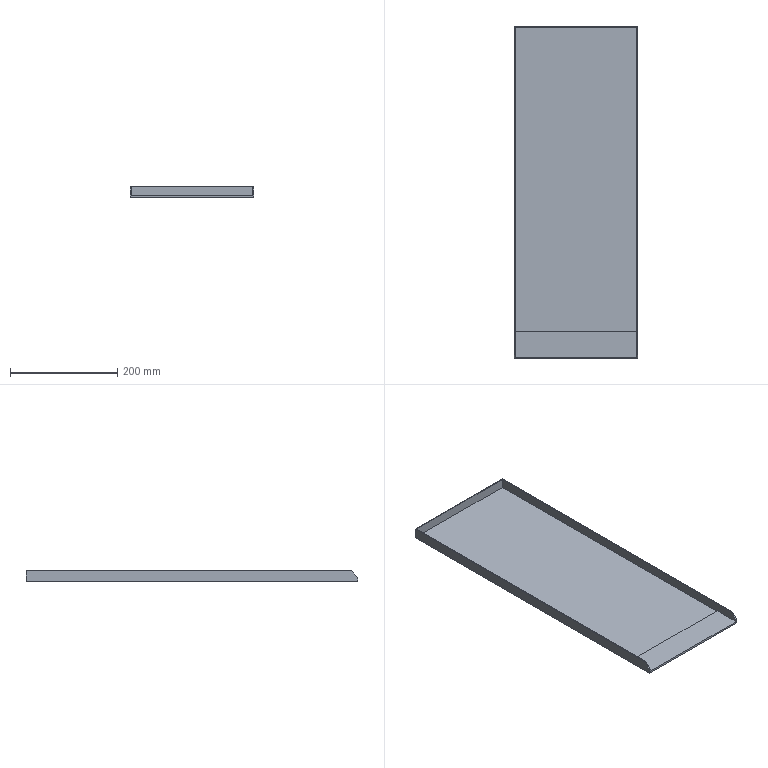Part | NX | features solid 2 | 1 solid | 14 faces | box 230 x 620 x 20 mm | volume 360238 mm3 | plane 14
STEP:
#1=CARTESIAN_POINT('',(360.,-460.,-313.));
#2=VERTEX_POINT('',#1);
#3=CARTESIAN_POINT('',(360.,-460.,-320.));
#4=VERTEX_POINT('',#3);
#5=CARTESIAN_POINT('',(360.,-460.,-318.));
#6=DIRECTION('',(0.,0.,-1.));
#7=VECTOR('',#6,1000.);
#8=LINE('',#5,#7);
#9=EDGE_CURVE('',#2,#4,#8,.T.);
#10=ORIENTED_EDGE('',*,*,#9,.F.);
#11=CARTESIAN_POINT('',(360.,-447.,-300.));
#12=VERTEX_POINT('',#11);
#13=CARTESIAN_POINT('',(360.,-445.,-298.));
#14=DIRECTION('',(0.,0.7071,0.7071));
#15=VECTOR('',#14,1000.);
#16=LINE('',#13,#15);
#17=EDGE_CURVE('',#2,#12,#16,.T.);
#18=ORIENTED_EDGE('',*,*,#17,.T.);
#19=CARTESIAN_POINT('',(360.,160.,-300.));
#20=VERTEX_POINT('',#19);
#21=CARTESIAN_POINT('',(360.,-70.,-300.));
#22=DIRECTION('',(0.,-1.,0.));
#23=VECTOR('',#22,1000.);
#24=LINE('',#21,#23);
#25=EDGE_CURVE('',#20,#12,#24,.T.);
#26=ORIENTED_EDGE('',*,*,#25,.F.);
#27=CARTESIAN_POINT('',(360.,160.,-320.));
#28=VERTEX_POINT('',#27);
#29=CARTESIAN_POINT('',(360.,160.,-318.));
#30=DIRECTION('',(0.,0.,-1.));
#31=VECTOR('',#30,1000.);
#32=LINE('',#29,#31);
#33=EDGE_CURVE('',#20,#28,#32,.T.);
#34=ORIENTED_EDGE('',*,*,#33,.T.);
#35=CARTESIAN_POINT('',(360.,-70.,-320.));
#36=DIRECTION('',(0.,1.,0.));
#37=VECTOR('',#36,1000.);
#38=LINE('',#35,#37);
#39=EDGE_CURVE('',#28,#4,#38,.F.);
#40=ORIENTED_EDGE('',*,*,#39,.T.);
#41=EDGE_LOOP('',(#10,#18,#26,#34,#40));
#42=FACE_BOUND('',#41,.T.);
#43=CARTESIAN_POINT('',(360.,-70.,-318.));
#44=DIRECTION('',(1.,0.,0.));
#45=DIRECTION('',(0.,0.,-1.));
#46=AXIS2_PLACEMENT_3D('',#43,#44,#45);
#47=PLANE('',#46);
#48=ADVANCED_FACE('',(#42),#47,.F.);
#49=CARTESIAN_POINT('',(590.,160.,-320.));
#50=VERTEX_POINT('',#49);
#51=CARTESIAN_POINT('',(-350.,160.,-320.));
#52=DIRECTION('',(1.,0.,0.));
#53=VECTOR('',#52,1000.);
#54=LINE('',#51,#53);
#55=EDGE_CURVE('',#50,#28,#54,.F.);
#56=ORIENTED_EDGE('',*,*,#55,.T.);
#57=ORIENTED_EDGE('',*,*,#33,.F.);
#58=CARTESIAN_POINT('',(590.,160.,-300.));
#59=VERTEX_POINT('',#58);
#60=CARTESIAN_POINT('',(-380.,160.,-300.));
#61=DIRECTION('',(1.,0.,0.));
#62=VECTOR('',#61,1000.);
#63=LINE('',#60,#62);
#64=EDGE_CURVE('',#20,#59,#63,.T.);
#65=ORIENTED_EDGE('',*,*,#64,.T.);
#66=CARTESIAN_POINT('',(590.,160.,-318.));
#67=DIRECTION('',(0.,0.,-1.));
#68=VECTOR('',#67,1000.);
#69=LINE('',#66,#68);
#70=EDGE_CURVE('',#59,#50,#69,.T.);
#71=ORIENTED_EDGE('',*,*,#70,.T.);
#72=EDGE_LOOP('',(#56,#57,#65,#71));
#73=FACE_BOUND('',#72,.T.);
#74=CARTESIAN_POINT('',(-350.,160.,-318.));
#75=DIRECTION('',(0.,-1.,0.));
#76=DIRECTION('',(0.,0.,-1.));
#77=AXIS2_PLACEMENT_3D('',#74,#75,#76);
#78=PLANE('',#77);
#79=ADVANCED_FACE('',(#73),#78,.F.);
#80=CARTESIAN_POINT('',(590.,-447.,-300.));
#81=VERTEX_POINT('',#80);
#82=CARTESIAN_POINT('',(590.,-15.,-300.));
#83=DIRECTION('',(0.,-1.,0.));
#84=VECTOR('',#83,1000.);
#85=LINE('',#82,#84);
#86=EDGE_CURVE('',#59,#81,#85,.T.);
#87=ORIENTED_EDGE('',*,*,#86,.T.);
#88=CARTESIAN_POINT('',(590.,-460.,-313.));
#89=VERTEX_POINT('',#88);
#90=CARTESIAN_POINT('',(590.,-460.,-313.));
#91=DIRECTION('',(0.,-0.7071,-0.7071));
#92=VECTOR('',#91,1000.);
#93=LINE('',#90,#92);
#94=EDGE_CURVE('',#81,#89,#93,.T.);
#95=ORIENTED_EDGE('',*,*,#94,.T.);
#96=CARTESIAN_POINT('',(590.,-460.,-320.));
#97=VERTEX_POINT('',#96);
#98=CARTESIAN_POINT('',(590.,-460.,-318.));
#99=DIRECTION('',(0.,0.,-1.));
#100=VECTOR('',#99,1000.);
#101=LINE('',#98,#100);
#102=EDGE_CURVE('',#89,#97,#101,.T.);
#103=ORIENTED_EDGE('',*,*,#102,.T.);
#104=CARTESIAN_POINT('',(590.,-70.,-320.));
#105=DIRECTION('',(0.,-1.,0.));
#106=VECTOR('',#105,1000.);
#107=LINE('',#104,#106);
#108=EDGE_CURVE('',#97,#50,#107,.F.);
#109=ORIENTED_EDGE('',*,*,#108,.T.);
#110=ORIENTED_EDGE('',*,*,#70,.F.);
#111=EDGE_LOOP('',(#87,#95,#103,#109,#110));
#112=FACE_BOUND('',#111,.T.);
#113=CARTESIAN_POINT('',(590.,-70.,-318.));
#114=DIRECTION('',(-1.,0.,0.));
#115=DIRECTION('',(0.,0.,1.));
#116=AXIS2_PLACEMENT_3D('',#113,#114,#115);
#117=PLANE('',#116);
#118=ADVANCED_FACE('',(#112),#117,.F.);
#119=CARTESIAN_POINT('',(362.,-460.,-316.));
#120=VERTEX_POINT('',#119);
#121=CARTESIAN_POINT('',(588.,-460.,-316.));
#122=VERTEX_POINT('',#121);
#123=CARTESIAN_POINT('',(362.,-460.,-316.));
#124=DIRECTION('',(-1.,0.,0.));
#125=VECTOR('',#124,1000.);
#126=LINE('',#123,#125);
#127=EDGE_CURVE('',#120,#122,#126,.F.);
#128=ORIENTED_EDGE('',*,*,#127,.F.);
#129=CARTESIAN_POINT('',(362.,-460.,-313.));
#130=VERTEX_POINT('',#129);
#131=CARTESIAN_POINT('',(362.,-460.,-318.));
#132=DIRECTION('',(0.,0.,-1.));
#133=VECTOR('',#132,1000.);
#134=LINE('',#131,#133);
#135=EDGE_CURVE('',#130,#120,#134,.T.);
#136=ORIENTED_EDGE('',*,*,#135,.F.);
#137=CARTESIAN_POINT('',(360.,-460.,-313.));
#138=DIRECTION('',(-1.,0.,0.));
#139=VECTOR('',#138,1000.);
#140=LINE('',#137,#139);
#141=EDGE_CURVE('',#130,#2,#140,.T.);
#142=ORIENTED_EDGE('',*,*,#141,.T.);
#143=ORIENTED_EDGE('',*,*,#9,.T.);
#144=CARTESIAN_POINT('',(-350.,-460.,-320.));
#145=DIRECTION('',(-1.,0.,0.));
#146=VECTOR('',#145,1000.);
#147=LINE('',#144,#146);
#148=EDGE_CURVE('',#4,#97,#147,.F.);
#149=ORIENTED_EDGE('',*,*,#148,.T.);
#150=ORIENTED_EDGE('',*,*,#102,.F.);
#151=CARTESIAN_POINT('',(588.,-460.,-313.));
#152=VERTEX_POINT('',#151);
#153=CARTESIAN_POINT('',(588.,-460.,-313.));
#154=DIRECTION('',(-1.,0.,0.));
#155=VECTOR('',#154,1000.);
#156=LINE('',#153,#155);
#157=EDGE_CURVE('',#89,#152,#156,.T.);
#158=ORIENTED_EDGE('',*,*,#157,.T.);
#159=CARTESIAN_POINT('',(588.,-460.,-318.));
#160=DIRECTION('',(0.,0.,-1.));
#161=VECTOR('',#160,1000.);
#162=LINE('',#159,#161);
#163=EDGE_CURVE('',#152,#122,#162,.T.);
#164=ORIENTED_EDGE('',*,*,#163,.T.);
#165=EDGE_LOOP('',(#128,#136,#142,#143,#149,#150,#158,#164));
#166=FACE_BOUND('',#165,.T.);
#167=CARTESIAN_POINT('',(-350.,-460.,-318.));
#168=DIRECTION('',(0.,1.,0.));
#169=DIRECTION('',(0.,0.,1.));
#170=AXIS2_PLACEMENT_3D('',#167,#168,#169);
#171=PLANE('',#170);
#172=ADVANCED_FACE('',(#166),#171,.F.);
#173=CARTESIAN_POINT('',(362.,-410.,-318.));
#174=VERTEX_POINT('',#173);
#175=CARTESIAN_POINT('',(588.,-410.,-318.));
#176=VERTEX_POINT('',#175);
#177=CARTESIAN_POINT('',(362.,-410.,-318.));
#178=DIRECTION('',(1.,0.,0.));
#179=VECTOR('',#178,1000.);
#180=LINE('',#177,#179);
#181=EDGE_CURVE('',#174,#176,#180,.T.);
#182=ORIENTED_EDGE('',*,*,#181,.T.);
#183=CARTESIAN_POINT('',(588.,158.,-318.));
#184=VERTEX_POINT('',#183);
#185=CARTESIAN_POINT('',(588.,-70.,-318.));
#186=DIRECTION('',(0.,1.,0.));
#187=VECTOR('',#186,1000.);
#188=LINE('',#185,#187);
#189=EDGE_CURVE('',#184,#176,#188,.F.);
#190=ORIENTED_EDGE('',*,*,#189,.F.);
#191=CARTESIAN_POINT('',(362.,158.,-318.));
#192=VERTEX_POINT('',#191);
#193=CARTESIAN_POINT('',(-350.,158.,-318.));
#194=DIRECTION('',(-1.,0.,0.));
#195=VECTOR('',#194,1000.);
#196=LINE('',#193,#195);
#197=EDGE_CURVE('',#192,#184,#196,.F.);
#198=ORIENTED_EDGE('',*,*,#197,.F.);
#199=CARTESIAN_POINT('',(362.,-70.,-318.));
#200=DIRECTION('',(0.,-1.,0.));
#201=VECTOR('',#200,1000.);
#202=LINE('',#199,#201);
#203=EDGE_CURVE('',#174,#192,#202,.F.);
#204=ORIENTED_EDGE('',*,*,#203,.F.);
#205=EDGE_LOOP('',(#182,#190,#198,#204));
#206=FACE_BOUND('',#205,.T.);
#207=CARTESIAN_POINT('',(-350.,-70.,-318.));
#208=DIRECTION('',(0.,0.,-1.));
#209=DIRECTION('',(-1.,0.,0.));
#210=AXIS2_PLACEMENT_3D('',#207,#208,#209);
#211=PLANE('',#210);
#212=ADVANCED_FACE('',(#206),#211,.F.);
#213=ORIENTED_EDGE('',*,*,#108,.F.);
#214=ORIENTED_EDGE('',*,*,#148,.F.);
#215=ORIENTED_EDGE('',*,*,#39,.F.);
#216=ORIENTED_EDGE('',*,*,#55,.F.);
#217=EDGE_LOOP('',(#213,#214,#215,#216));
#218=FACE_BOUND('',#217,.T.);
#219=CARTESIAN_POINT('',(-350.,-70.,-320.));
#220=DIRECTION('',(0.,0.,-1.));
#221=DIRECTION('',(-1.,0.,0.));
#222=AXIS2_PLACEMENT_3D('',#219,#220,#221);
#223=PLANE('',#222);
#224=ADVANCED_FACE('',(#218),#223,.T.);
#225=CARTESIAN_POINT('',(588.,-447.,-300.));
#226=VERTEX_POINT('',#225);
#227=CARTESIAN_POINT('',(588.,158.,-300.));
#228=VERTEX_POINT('',#227);
#229=CARTESIAN_POINT('',(588.,-70.,-300.));
#230=DIRECTION('',(0.,1.,0.));
#231=VECTOR('',#230,1000.);
#232=LINE('',#229,#231);
#233=EDGE_CURVE('',#226,#228,#232,.T.);
#234=ORIENTED_EDGE('',*,*,#233,.F.);
#235=CARTESIAN_POINT('',(-380.,-447.,-300.));
#236=DIRECTION('',(1.,0.,0.));
#237=VECTOR('',#236,1000.);
#238=LINE('',#235,#237);
#239=EDGE_CURVE('',#226,#81,#238,.T.);
#240=ORIENTED_EDGE('',*,*,#239,.T.);
#241=ORIENTED_EDGE('',*,*,#86,.F.);
#242=ORIENTED_EDGE('',*,*,#64,.F.);
#243=ORIENTED_EDGE('',*,*,#25,.T.);
#244=CARTESIAN_POINT('',(362.,-447.,-300.));
#245=VERTEX_POINT('',#244);
#246=CARTESIAN_POINT('',(-380.,-447.,-300.));
#247=DIRECTION('',(1.,0.,0.));
#248=VECTOR('',#247,1000.);
#249=LINE('',#246,#248);
#250=EDGE_CURVE('',#12,#245,#249,.T.);
#251=ORIENTED_EDGE('',*,*,#250,.T.);
#252=CARTESIAN_POINT('',(362.,158.,-300.));
#253=VERTEX_POINT('',#252);
#254=CARTESIAN_POINT('',(362.,-70.,-300.));
#255=DIRECTION('',(0.,-1.,0.));
#256=VECTOR('',#255,1000.);
#257=LINE('',#254,#256);
#258=EDGE_CURVE('',#253,#245,#257,.T.);
#259=ORIENTED_EDGE('',*,*,#258,.F.);
#260=CARTESIAN_POINT('',(-350.,158.,-300.));
#261=DIRECTION('',(-1.,0.,0.));
#262=VECTOR('',#261,1000.);
#263=LINE('',#260,#262);
#264=EDGE_CURVE('',#228,#253,#263,.T.);
#265=ORIENTED_EDGE('',*,*,#264,.F.);
#266=EDGE_LOOP('',(#234,#240,#241,#242,#243,#251,#259,#265));
#267=FACE_BOUND('',#266,.T.);
#268=CARTESIAN_POINT('',(-380.,-15.,-300.));
#269=DIRECTION('',(0.,0.,1.));
#270=DIRECTION('',(1.,0.,0.));
#271=AXIS2_PLACEMENT_3D('',#268,#269,#270);
#272=PLANE('',#271);
#273=ADVANCED_FACE('',(#267),#272,.T.);
#274=CARTESIAN_POINT('',(362.,-410.,-316.));
#275=VERTEX_POINT('',#274);
#276=CARTESIAN_POINT('',(362.,-410.,-318.));
#277=DIRECTION('',(0.,0.,1.));
#278=VECTOR('',#277,1000.);
#279=LINE('',#276,#278);
#280=EDGE_CURVE('',#174,#275,#279,.T.);
#281=ORIENTED_EDGE('',*,*,#280,.F.);
#282=ORIENTED_EDGE('',*,*,#203,.T.);
#283=CARTESIAN_POINT('',(362.,158.,-318.));
#284=DIRECTION('',(0.,0.,-1.));
#285=VECTOR('',#284,1000.);
#286=LINE('',#283,#285);
#287=EDGE_CURVE('',#253,#192,#286,.T.);
#288=ORIENTED_EDGE('',*,*,#287,.F.);
#289=ORIENTED_EDGE('',*,*,#258,.T.);
#290=CARTESIAN_POINT('',(362.,-267.5,-120.5));
#291=DIRECTION('',(0.,-0.7071,-0.7071));
#292=VECTOR('',#291,1000.);
#293=LINE('',#290,#292);
#294=EDGE_CURVE('',#245,#130,#293,.T.);
#295=ORIENTED_EDGE('',*,*,#294,.T.);
#296=ORIENTED_EDGE('',*,*,#135,.T.);
#297=CARTESIAN_POINT('',(362.,-410.,-316.));
#298=DIRECTION('',(0.,1.,0.));
#299=VECTOR('',#298,1000.);
#300=LINE('',#297,#299);
#301=EDGE_CURVE('',#275,#120,#300,.F.);
#302=ORIENTED_EDGE('',*,*,#301,.F.);
#303=EDGE_LOOP('',(#281,#282,#288,#289,#295,#296,#302));
#304=FACE_BOUND('',#303,.T.);
#305=CARTESIAN_POINT('',(362.,-70.,-318.));
#306=DIRECTION('',(1.,0.,0.));
#307=DIRECTION('',(0.,0.,-1.));
#308=AXIS2_PLACEMENT_3D('',#305,#306,#307);
#309=PLANE('',#308);
#310=ADVANCED_FACE('',(#304),#309,.T.);
#311=ORIENTED_EDGE('',*,*,#287,.T.);
#312=ORIENTED_EDGE('',*,*,#197,.T.);
#313=CARTESIAN_POINT('',(588.,158.,-318.));
#314=DIRECTION('',(0.,0.,-1.));
#315=VECTOR('',#314,1000.);
#316=LINE('',#313,#315);
#317=EDGE_CURVE('',#228,#184,#316,.T.);
#318=ORIENTED_EDGE('',*,*,#317,.F.);
#319=ORIENTED_EDGE('',*,*,#264,.T.);
#320=EDGE_LOOP('',(#311,#312,#318,#319));
#321=FACE_BOUND('',#320,.T.);
#322=CARTESIAN_POINT('',(-350.,158.,-318.));
#323=DIRECTION('',(0.,-1.,0.));
#324=DIRECTION('',(0.,0.,-1.));
#325=AXIS2_PLACEMENT_3D('',#322,#323,#324);
#326=PLANE('',#325);
#327=ADVANCED_FACE('',(#321),#326,.T.);
#328=CARTESIAN_POINT('',(588.,-410.,-316.));
#329=VERTEX_POINT('',#328);
#330=CARTESIAN_POINT('',(588.,-410.,-318.));
#331=DIRECTION('',(0.,0.,1.));
#332=VECTOR('',#331,1000.);
#333=LINE('',#330,#332);
#334=EDGE_CURVE('',#176,#329,#333,.T.);
#335=ORIENTED_EDGE('',*,*,#334,.T.);
#336=CARTESIAN_POINT('',(588.,-410.,-316.));
#337=DIRECTION('',(0.,1.,0.));
#338=VECTOR('',#337,1000.);
#339=LINE('',#336,#338);
#340=EDGE_CURVE('',#329,#122,#339,.F.);
#341=ORIENTED_EDGE('',*,*,#340,.T.);
#342=ORIENTED_EDGE('',*,*,#163,.F.);
#343=CARTESIAN_POINT('',(588.,-267.5,-120.5));
#344=DIRECTION('',(0.,0.7071,0.7071));
#345=VECTOR('',#344,1000.);
#346=LINE('',#343,#345);
#347=EDGE_CURVE('',#152,#226,#346,.T.);
#348=ORIENTED_EDGE('',*,*,#347,.T.);
#349=ORIENTED_EDGE('',*,*,#233,.T.);
#350=ORIENTED_EDGE('',*,*,#317,.T.);
#351=ORIENTED_EDGE('',*,*,#189,.T.);
#352=EDGE_LOOP('',(#335,#341,#342,#348,#349,#350,#351));
#353=FACE_BOUND('',#352,.T.);
#354=CARTESIAN_POINT('',(588.,-70.,-318.));
#355=DIRECTION('',(-1.,0.,0.));
#356=DIRECTION('',(0.,0.,1.));
#357=AXIS2_PLACEMENT_3D('',#354,#355,#356);
#358=PLANE('',#357);
#359=ADVANCED_FACE('',(#353),#358,.T.);
#360=ORIENTED_EDGE('',*,*,#94,.F.);
#361=ORIENTED_EDGE('',*,*,#239,.F.);
#362=ORIENTED_EDGE('',*,*,#347,.F.);
#363=ORIENTED_EDGE('',*,*,#157,.F.);
#364=EDGE_LOOP('',(#360,#361,#362,#363));
#365=FACE_BOUND('',#364,.T.);
#366=CARTESIAN_POINT('',(-350.,-460.,-313.));
#367=DIRECTION('',(0.,-0.7071,0.7071));
#368=DIRECTION('',(0.,-0.7071,-0.7071));
#369=AXIS2_PLACEMENT_3D('',#366,#367,#368);
#370=PLANE('',#369);
#371=ADVANCED_FACE('',(#365),#370,.T.);
#372=ORIENTED_EDGE('',*,*,#17,.F.);
#373=ORIENTED_EDGE('',*,*,#141,.F.);
#374=ORIENTED_EDGE('',*,*,#294,.F.);
#375=ORIENTED_EDGE('',*,*,#250,.F.);
#376=EDGE_LOOP('',(#372,#373,#374,#375));
#377=FACE_BOUND('',#376,.T.);
#378=CARTESIAN_POINT('',(360.,-445.,-298.));
#379=DIRECTION('',(0.,-0.7071,0.7071));
#380=DIRECTION('',(0.,-0.7071,-0.7071));
#381=AXIS2_PLACEMENT_3D('',#378,#379,#380);
#382=PLANE('',#381);
#383=ADVANCED_FACE('',(#377),#382,.T.);
#384=ORIENTED_EDGE('',*,*,#334,.F.);
#385=ORIENTED_EDGE('',*,*,#181,.F.);
#386=ORIENTED_EDGE('',*,*,#280,.T.);
#387=CARTESIAN_POINT('',(362.,-410.,-316.));
#388=DIRECTION('',(-1.,0.,0.));
#389=VECTOR('',#388,1000.);
#390=LINE('',#387,#389);
#391=EDGE_CURVE('',#275,#329,#390,.F.);
#392=ORIENTED_EDGE('',*,*,#391,.T.);
#393=EDGE_LOOP('',(#384,#385,#386,#392));
#394=FACE_BOUND('',#393,.T.);
#395=CARTESIAN_POINT('',(362.,-410.,-318.));
#396=DIRECTION('',(0.,1.,0.));
#397=DIRECTION('',(1.,0.,0.));
#398=AXIS2_PLACEMENT_3D('',#395,#396,#397);
#399=PLANE('',#398);
#400=ADVANCED_FACE('',(#394),#399,.T.);
#401=ORIENTED_EDGE('',*,*,#127,.T.);
#402=ORIENTED_EDGE('',*,*,#340,.F.);
#403=ORIENTED_EDGE('',*,*,#391,.F.);
#404=ORIENTED_EDGE('',*,*,#301,.T.);
#405=EDGE_LOOP('',(#401,#402,#403,#404));
#406=FACE_BOUND('',#405,.T.);
#407=CARTESIAN_POINT('',(362.,-410.,-316.));
#408=DIRECTION('',(0.,0.,-1.));
#409=DIRECTION('',(-1.,0.,0.));
#410=AXIS2_PLACEMENT_3D('',#407,#408,#409);
#411=PLANE('',#410);
#412=ADVANCED_FACE('',(#406),#411,.F.);
#413=CLOSED_SHELL('',(#48,#79,#118,#172,#212,#224,#273,#310,#327,#359,#371,#383,#400,#412));
#414=MANIFOLD_SOLID_BREP('',#413);
#415=(LENGTH_UNIT()NAMED_UNIT(*)SI_UNIT(.MILLI.,.METRE.));
#416=UNCERTAINTY_MEASURE_WITH_UNIT(LENGTH_MEASURE(0.00001),#415,'','');
#417=(NAMED_UNIT(*)PLANE_ANGLE_UNIT()SI_UNIT($,.RADIAN.));
#418=(NAMED_UNIT(*)SI_UNIT($,.STERADIAN.)SOLID_ANGLE_UNIT());
#419=(GEOMETRIC_REPRESENTATION_CONTEXT(3)GLOBAL_UNCERTAINTY_ASSIGNED_CONTEXT((#416))GLOBAL_UNIT_ASSIGNED_CONTEXT((#415,#417,#418))REPRESENTATION_CONTEXT('',''));
#420=ADVANCED_BREP_SHAPE_REPRESENTATION('',(#414),#419);